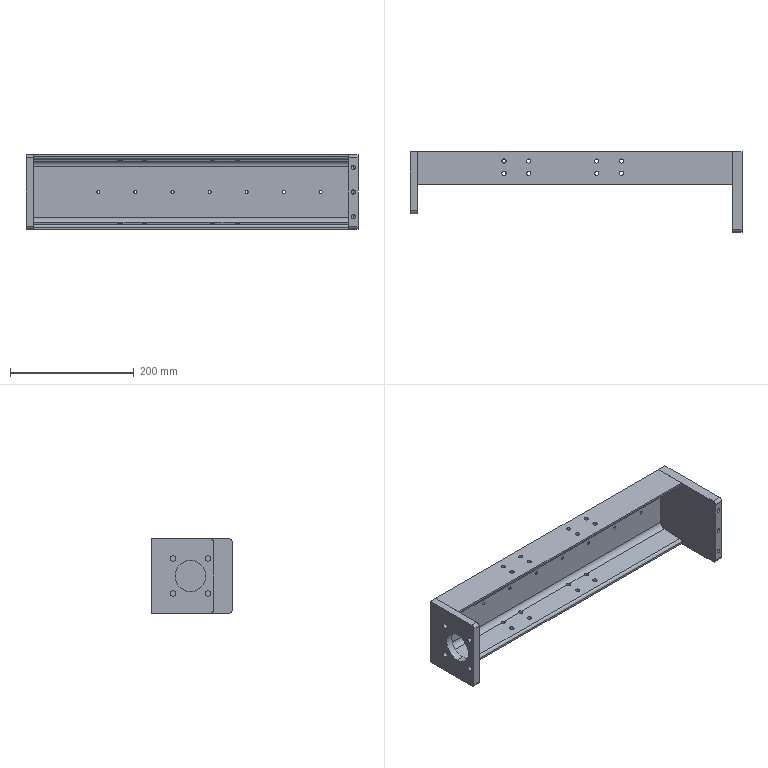Part | SolidWorks | features HoleWzd 4, Fillet 2, ICE 2, Cut 1, LPattern 1, WeldMemberFeat 1, WeldmentFeature 1 | 3 solids | 98 faces | box 537 x 130 x 120 mm | volume 1117670 mm3 | cylinder 70 | plane 22 | cone 6 | commonest cylinder face diameters 6.8 x38 5 x14 9 x10 10 x4 18 x2 50 x2